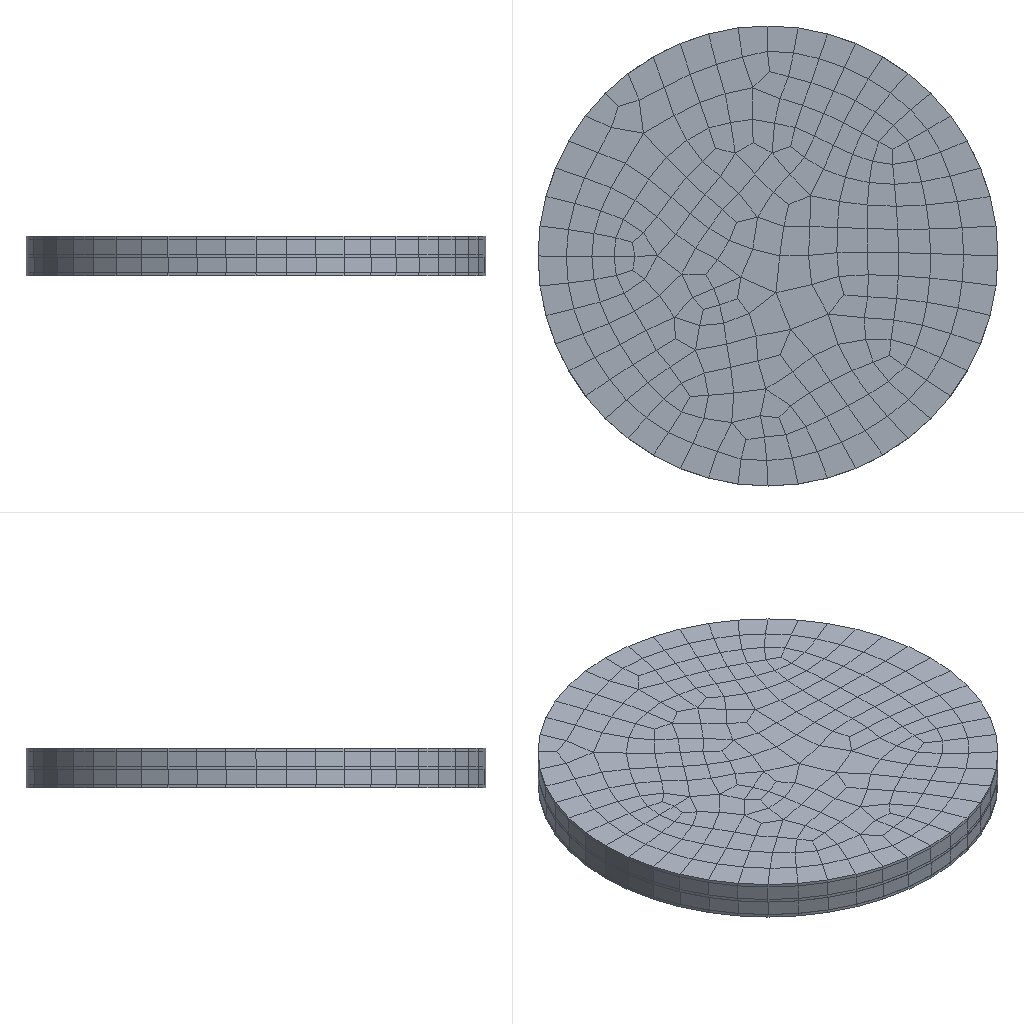Simulation study | abaqus
Set-up summary:
category,name,step,type,value,unit,region
solver,abaqus
solver,version,,,Abaqus/Standard 2020
units,not stated in the deck,,not stated
analysis,deck,,static,static
load_step,Step-1,Step-1,static
load_step,requested,,,1
mesh,nodes,,,2754
mesh,elements,,,1252
element_type,C3D8E,,solid,1252
load,load commands in deck,,count,1
bc,support commands in deck,,count,3
material,MATERIAL-1,,in results
check,setup vs results,,match,"per instance, exact: element labels, types and connectivity; labels of the nodes the elements use; coordinates of those nodes at SINGLE_PRECISION in 2 of 5 instance(s)"
Abaqus input file, long lists of numbers shortened:
*Heading
** Job name: Job-1 Model name: Model-1
** Generated by: Abaqus/CAE 2020
*Preprint, echo=NO, model=NO, history=NO, contact=NO
**
** PARTS
**
*Part, name=work-1
*Node
      1,   7.25,   -1.921,  0.1
      2,   6.937,  -2.85,  0.1
** (550 more lines like these left out)
*Element, type=C3D8E
  1, 402, 372, 341, 396, 126,  96,  65, 120
  2, 285, 325, 355, 284,   9,  49,  79,   8
** (249 more lines like these left out)
*Nset, nset=Set-1, generate
   1,  552,    1
*Elset, elset=Set-1, generate
   1,  251,    1
*Orientation, name=Ori-1
1., 0., 0., 0., 1., 0.
1, 0.
** Section: Section-1
*Solid Section, elset=Set-1, orientation=Ori-1, material=Material-1
,
*End Part
**
*Part, name=work-2
*Node
      1,   7.244,   -1.941,   1.2
      2,    6.929,  -2.87,   1.2
** (546 more lines like these left out)
*Element, type=C3D8E
  1, 401, 370, 338, 391, 127,  96,  64, 117
  2, 283, 323, 352, 282,   9,  49,  78,   8
** (247 more lines like these left out)
*Nset, nset=Set-1, generate
   1,  548,    1
*Elset, elset=Set-1, generate
   1,  249,    1
*Orientation, name=Ori-1
1., 0., 0., 0., 1., 0.
1, 0.
** Section: Section-1
*Solid Section, elset=Set-1, orientation=Ori-1, material=Material-1
,
*End Part
**
*Part, name=work-3
*Node
      1,   7.244,   -1.941,  0.6
      2,    6.929,  -2.87,  0.6
** (560 more lines like these left out)
*Element, type=C3D8E
  1, 408, 377, 345, 398, 127,  96,  64, 117
  2, 290, 330, 359, 289,   9,  49,  78,   8
** (254 more lines like these left out)
*Nset, nset=Set-1, generate
   1,  562,    1
*Elset, elset=Set-1, generate
   1,  256,    1
*Orientation, name=Ori-1
1., 0., 0., 0., 1., 0.
1, 0.
** Section: Section-1
*Solid Section, elset=Set-1, orientation=Ori-1, material=Material-1
,
*End Part
**
*Part, name=work-4
*Node
      1,   7.244,   -1.941,  0.7
      2,    6.929,  -2.87,  0.7
** (544 more lines like these left out)
*Element, type=C3D8E
  1, 400, 369, 337, 390, 127,  96,  64, 117
  2, 282, 322, 351, 281,   9,  49,  78,   8
** (246 more lines like these left out)
*Nset, nset=Set-1, generate
   1,  546,    1
*Elset, elset=Set-1, generate
   1,  248,    1
*Orientation, name=Ori-1
1., 0., 0., 0., 1., 0.
1, 0.
** Section: Section-1
*Solid Section, elset=Set-1, orientation=Ori-1, material=Material-1
,
*End Part
**
*Part, name=work-5
*Node
      1,   7.244,   -1.941,           0.
      2,    6.929,  -2.87,           0.
** (544 more lines like these left out)
*Element, type=C3D8E
  1, 400, 369, 337, 390, 127,  96,  64, 117
  2, 282, 322, 351, 281,   9,  49,  78,   8
** (246 more lines like these left out)
*Nset, nset=Set-1, generate
   1,  546,    1
*Elset, elset=Set-1, generate
   1,  248,    1
*Orientation, name=Ori-2
1., 0., 0., 0., 1., 0.
1, 0.
** Section: Section-1
*Solid Section, elset=Set-1, orientation=Ori-2, material=Material-1
,
*End Part
**
**
** ASSEMBLY
**
*Assembly, name=Assembly
**
*Instance, name=work-1-1, part=work-1
*End Instance
**
*Instance, name=work-2-1, part=work-2
*End Instance
**
*Instance, name=work-3-1, part=work-3
*End Instance
**
*Instance, name=work-4-1, part=work-4
*End Instance
**
*Instance, name=work-5-1, part=work-5
*End Instance
**
*Nset, nset=Set-1, instance=work-2-1, generate
 275,  548,    1
*Elset, elset=Set-1, instance=work-2-1, generate
   1,  249,    1
*Nset, nset=Set-2, instance=work-2-1, generate
 275,  548,    1
*Elset, elset=Set-2, instance=work-2-1, generate
   1,  249,    1
*Nset, nset=Set-3, instance=work-4-1, generate
   1,  273,    1
*Elset, elset=Set-3, instance=work-4-1, generate
   1,  248,    1
*Nset, nset=Set-4, instance=work-1-1, generate
 277,  552,    1
*Elset, elset=Set-4, instance=work-1-1, generate
   1,  251,    1
*Elset, elset=_Surf-9_S2, internal, instance=work-5-1, generate
   1,  248,    1
*Surface, type=ELEMENT, name=Surf-9
_Surf-9_S2, S2
*Elset, elset=_m_Surf-1_S2, internal, instance=work-2-1, generate
   1,  249,    1
*Surface, type=ELEMENT, name=m_Surf-1
_m_Surf-1_S2, S2
*Elset, elset=_m_Surf-3_S2, internal, instance=work-4-1, generate
   1,  248,    1
*Surface, type=ELEMENT, name=m_Surf-3
_m_Surf-3_S2, S2
*Elset, elset=_m_Surf-5_S2, internal, instance=work-3-1, generate
   1,  256,    1
*Surface, type=ELEMENT, name=m_Surf-5
_m_Surf-5_S2, S2
*Elset, elset=_m_Surf-7_S2, internal, instance=work-1-1, generate
   1,  251,    1
*Surface, type=ELEMENT, name=m_Surf-7
_m_Surf-7_S2, S2
*Elset, elset=_s_Surf-1_S1, internal, instance=work-4-1, generate
   1,  248,    1
*Surface, type=ELEMENT, name=s_Surf-1
_s_Surf-1_S1, S1
*Elset, elset=_s_Surf-3_S1, internal, instance=work-3-1, generate
   1,  256,    1
*Surface, type=ELEMENT, name=s_Surf-3
_s_Surf-3_S1, S1
*Elset, elset=_s_Surf-5_S1, internal, instance=work-1-1, generate
   1,  251,    1
*Surface, type=ELEMENT, name=s_Surf-5
_s_Surf-5_S1, S1
*Elset, elset=_s_Surf-7_S1, internal, instance=work-5-1, generate
   1,  248,    1
*Surface, type=ELEMENT, name=s_Surf-7
_s_Surf-7_S1, S1
** Constraint: Constraint-1
*Tie, name=Constraint-1, adjust=yes
s_Surf-1, m_Surf-1
** Constraint: Constraint-2
*Tie, name=Constraint-2, adjust=yes
s_Surf-3, m_Surf-3
** Constraint: Constraint-3
*Tie, name=Constraint-3, adjust=yes
s_Surf-5, m_Surf-5
** Constraint: Constraint-4
*Tie, name=Constraint-4, adjust=yes
s_Surf-7, m_Surf-7
*End Assembly
*Amplitude, name=Amp-1
             0.,              0.,              1.,              1.
**
** MATERIALS
**
*Material, name=Material-1
*Dielectric, type=ORTHO
 8.107e-09,        0., 7.346e-09
*Elastic, type=ORTHOTROPIC
121000., 75400.,121000., 75200., 75200.,111000., 21100., 21100.
 21100.,
*Piezoelectric
0.,   0.,   0.,   0., 12.3,   0.,   0.,   0.
   0.,   0.,   0., 12.7, -5.4, -5.4, 15.8,   0.
   0.,   0.
** ----------------------------------------------------------------
**
** STEP: Step-1
**
*Step, name=Step-1, nlgeom=YES, inc=1000
*Static, stabilize=0.0002, allsdtol=0.05, continue=NO
0.01, 1., 1e-05, 1.
**
** BOUNDARY CONDITIONS
**
** Name: BC-1 Type: 对称/反对称/完全固定
*Boundary
Set-1, ENCASTRE
** Name: BC-2 Type: 电势
*Boundary
Set-3, 9, 9
** Name: BC-2-Copy Type: 电势
*Boundary
Set-4, 9, 9
**
** LOADS
**
** Name: Load-1   Type: Pressure
*Dsload, amplitude=Amp-1
Surf-9, P, 0.1274
**
** OUTPUT REQUESTS
**
*Restart, write, frequency=0
**
** FIELD OUTPUT: F-Output-1
**
*Output, field
*Node Output
CF, EPOT, RF, RM, RT, U, V
*Element Output, directions=YES
E, LE, MISES, MISESMAX, PE, PEEQ, PEMAG, S, TSHR
*Contact Output
CDISP, CSTRESS
**
** HISTORY OUTPUT: H-Output-1
**
*Output, history, variable=PRESELECT
*End Step
Results summary:
result,step,,completed,increments=11 time=1.0/1.0
result,analysis,,,static
result,last_loadstep,,,1
result,primary field,,,U
result,reaction total,,FX,0.0,model units
result,reaction total,,FY,-0.0,model units
result,reaction total,,FZ,-22.449,model units